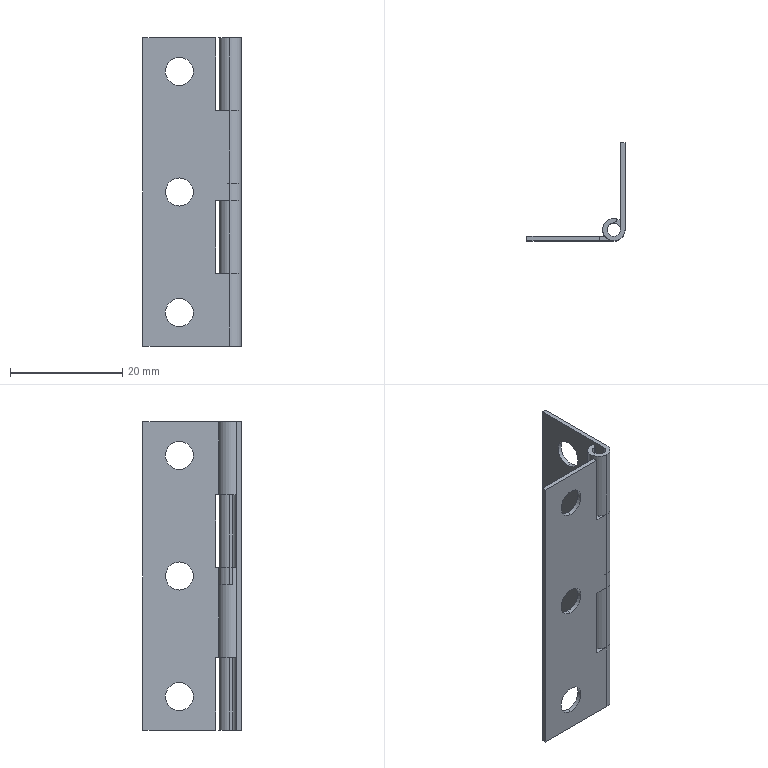Part | SolidWorks | features BaseBody 2, MoveFace 2, CoordSys 1 | 2 solids | 60 faces | box 17.5 x 17.5 x 55 mm | volume 1534 mm3 | cylinder 36 | plane 24 | commonest cylinder face diameters 2.4 x12 4 x12 5 x12